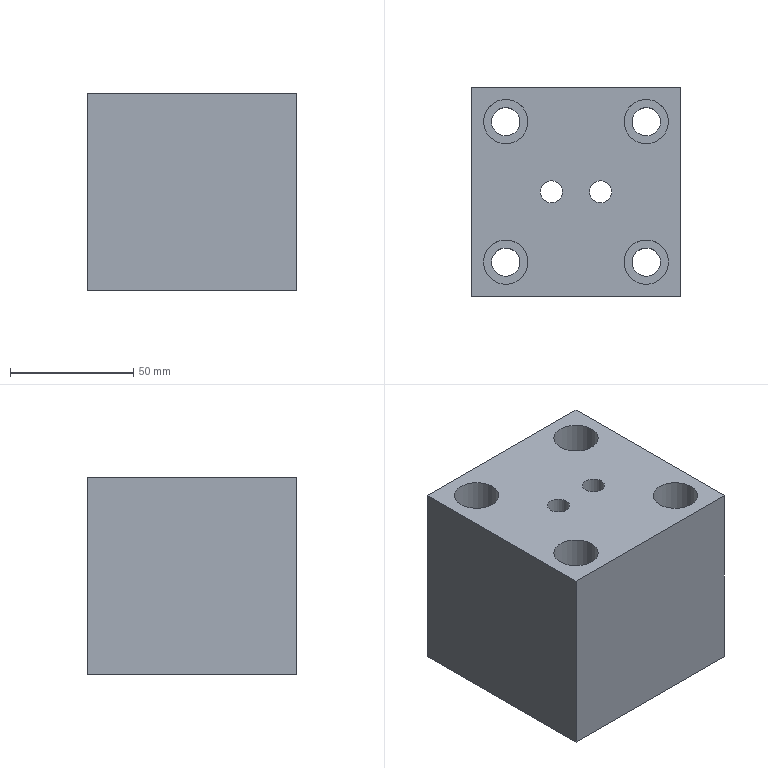Part | STEP file | lll_id4374_x_t | 1 solid | 24 faces | box 85 x 85 x 80 mm | volume 511038 mm3 | plane 12 | cylinder 12 | commonest cylinder face diameters 11.509 x4 18.008 x4 9 x2 14 x2
STEP:
#1=CARTESIAN_POINT('',(1584.69,-336.,-370.));
#2=VERTEX_POINT('',#1);
#3=CARTESIAN_POINT('',(1578.935,-336.,-370.));
#4=DIRECTION('',(0.,0.,1.));
#5=DIRECTION('',(1.,0.,0.));
#6=AXIS2_PLACEMENT_3D('',#3,#4,#5);
#7=CIRCLE('',#6,5.755);
#8=EDGE_CURVE('',#2,#2,#7,.T.);
#9=ORIENTED_EDGE('',*,*,#8,.T.);
#10=EDGE_LOOP('',(#9));
#11=FACE_BOUND('',#10,.T.);
#12=CARTESIAN_POINT('',(1584.69,-279.,-370.));
#13=VERTEX_POINT('',#12);
#14=CARTESIAN_POINT('',(1578.935,-279.,-370.));
#15=DIRECTION('',(0.,0.,1.));
#16=DIRECTION('',(1.,0.,0.));
#17=AXIS2_PLACEMENT_3D('',#14,#15,#16);
#18=CIRCLE('',#17,5.755);
#19=EDGE_CURVE('',#13,#13,#18,.T.);
#20=ORIENTED_EDGE('',*,*,#19,.T.);
#21=EDGE_LOOP('',(#20));
#22=FACE_BOUND('',#21,.T.);
#23=CARTESIAN_POINT('',(1527.69,-336.,-370.));
#24=VERTEX_POINT('',#23);
#25=CARTESIAN_POINT('',(1521.935,-336.,-370.));
#26=DIRECTION('',(0.,0.,1.));
#27=DIRECTION('',(1.,0.,0.));
#28=AXIS2_PLACEMENT_3D('',#25,#26,#27);
#29=CIRCLE('',#28,5.755);
#30=EDGE_CURVE('',#24,#24,#29,.T.);
#31=ORIENTED_EDGE('',*,*,#30,.T.);
#32=EDGE_LOOP('',(#31));
#33=FACE_BOUND('',#32,.T.);
#34=CARTESIAN_POINT('',(1527.69,-279.,-370.));
#35=VERTEX_POINT('',#34);
#36=CARTESIAN_POINT('',(1521.935,-279.,-370.));
#37=DIRECTION('',(0.,0.,1.));
#38=DIRECTION('',(1.,0.,0.));
#39=AXIS2_PLACEMENT_3D('',#36,#37,#38);
#40=CIRCLE('',#39,5.755);
#41=EDGE_CURVE('',#35,#35,#40,.T.);
#42=ORIENTED_EDGE('',*,*,#41,.T.);
#43=EDGE_LOOP('',(#42));
#44=FACE_BOUND('',#43,.T.);
#45=CARTESIAN_POINT('',(1592.935,-350.,-370.));
#46=VERTEX_POINT('',#45);
#47=CARTESIAN_POINT('',(1592.935,-265.,-370.));
#48=VERTEX_POINT('',#47);
#49=CARTESIAN_POINT('',(1592.935,0.,-370.));
#50=DIRECTION('',(0.,1.,0.));
#51=VECTOR('',#50,1.);
#52=LINE('',#49,#51);
#53=EDGE_CURVE('',#46,#48,#52,.T.);
#54=ORIENTED_EDGE('',*,*,#53,.F.);
#55=CARTESIAN_POINT('',(1507.935,-350.,-370.));
#56=VERTEX_POINT('',#55);
#57=CARTESIAN_POINT('',(1550.435,-350.,-370.));
#58=DIRECTION('',(-1.,0.,0.));
#59=VECTOR('',#58,1.);
#60=LINE('',#57,#59);
#61=EDGE_CURVE('',#46,#56,#60,.T.);
#62=ORIENTED_EDGE('',*,*,#61,.T.);
#63=CARTESIAN_POINT('',(1507.935,-265.,-370.));
#64=VERTEX_POINT('',#63);
#65=CARTESIAN_POINT('',(1507.935,0.,-370.));
#66=DIRECTION('',(0.,-1.,0.));
#67=VECTOR('',#66,1.);
#68=LINE('',#65,#67);
#69=EDGE_CURVE('',#64,#56,#68,.T.);
#70=ORIENTED_EDGE('',*,*,#69,.F.);
#71=CARTESIAN_POINT('',(2132.435,-265.,-370.));
#72=DIRECTION('',(-1.,0.,0.));
#73=VECTOR('',#72,1.);
#74=LINE('',#71,#73);
#75=EDGE_CURVE('',#48,#64,#74,.T.);
#76=ORIENTED_EDGE('',*,*,#75,.F.);
#77=EDGE_LOOP('',(#54,#62,#70,#76));
#78=FACE_BOUND('',#77,.T.);
#79=CARTESIAN_POINT('',(1567.435,-307.5,-370.));
#80=VERTEX_POINT('',#79);
#81=CARTESIAN_POINT('',(1560.435,-307.5,-370.));
#82=DIRECTION('',(0.,0.,1.));
#83=DIRECTION('',(1.,0.,0.));
#84=AXIS2_PLACEMENT_3D('',#81,#82,#83);
#85=CIRCLE('',#84,7.);
#86=EDGE_CURVE('',#80,#80,#85,.T.);
#87=ORIENTED_EDGE('',*,*,#86,.T.);
#88=EDGE_LOOP('',(#87));
#89=FACE_BOUND('',#88,.T.);
#90=CARTESIAN_POINT('',(1547.435,-307.5,-370.));
#91=VERTEX_POINT('',#90);
#92=CARTESIAN_POINT('',(1540.435,-307.5,-370.));
#93=DIRECTION('',(0.,0.,-1.));
#94=DIRECTION('',(1.,0.,0.));
#95=AXIS2_PLACEMENT_3D('',#92,#93,#94);
#96=CIRCLE('',#95,7.);
#97=EDGE_CURVE('',#91,#91,#96,.T.);
#98=ORIENTED_EDGE('',*,*,#97,.F.);
#99=EDGE_LOOP('',(#98));
#100=FACE_BOUND('',#99,.T.);
#101=CARTESIAN_POINT('',(2132.435,0.,-370.));
#102=DIRECTION('',(0.,0.,1.));
#103=DIRECTION('',(1.,0.,0.));
#104=AXIS2_PLACEMENT_3D('',#101,#102,#103);
#105=PLANE('',#104);
#106=ADVANCED_FACE('',(#11,#22,#33,#44,#78,#89,#100),#105,.F.);
#107=CARTESIAN_POINT('',(1535.935,-307.5,-290.));
#108=VERTEX_POINT('',#107);
#109=CARTESIAN_POINT('',(1540.435,-307.5,-290.));
#110=DIRECTION('',(0.,0.,-1.));
#111=DIRECTION('',(-1.,0.,0.));
#112=AXIS2_PLACEMENT_3D('',#109,#110,#111);
#113=CIRCLE('',#112,4.5);
#114=EDGE_CURVE('',#108,#108,#113,.T.);
#115=ORIENTED_EDGE('',*,*,#114,.F.);
#116=EDGE_LOOP('',(#115));
#117=FACE_BOUND('',#116,.T.);
#118=CARTESIAN_POINT('',(1535.935,-307.5,-300.));
#119=VERTEX_POINT('',#118);
#120=CARTESIAN_POINT('',(1540.435,-307.5,-300.));
#121=DIRECTION('',(0.,0.,-1.));
#122=DIRECTION('',(-1.,0.,0.));
#123=AXIS2_PLACEMENT_3D('',#120,#121,#122);
#124=CIRCLE('',#123,4.5);
#125=EDGE_CURVE('',#119,#119,#124,.T.);
#126=ORIENTED_EDGE('',*,*,#125,.T.);
#127=EDGE_LOOP('',(#126));
#128=FACE_BOUND('',#127,.T.);
#129=CARTESIAN_POINT('',(1540.435,-307.5,-510.));
#130=DIRECTION('',(0.,0.,1.));
#131=DIRECTION('',(1.,0.,0.));
#132=AXIS2_PLACEMENT_3D('',#129,#130,#131);
#133=CYLINDRICAL_SURFACE('',#132,4.5);
#134=ADVANCED_FACE('',(#117,#128),#133,.F.);
#135=ORIENTED_EDGE('',*,*,#114,.T.);
#136=EDGE_LOOP('',(#135));
#137=FACE_BOUND('',#136,.T.);
#138=CARTESIAN_POINT('',(1592.935,-265.,-290.));
#139=VERTEX_POINT('',#138);
#140=CARTESIAN_POINT('',(1592.935,-350.,-290.));
#141=VERTEX_POINT('',#140);
#142=CARTESIAN_POINT('',(1592.935,-87.5,-290.));
#143=DIRECTION('',(0.,-1.,0.));
#144=VECTOR('',#143,1.);
#145=LINE('',#142,#144);
#146=EDGE_CURVE('',#139,#141,#145,.T.);
#147=ORIENTED_EDGE('',*,*,#146,.F.);
#148=CARTESIAN_POINT('',(1507.935,-265.,-290.));
#149=VERTEX_POINT('',#148);
#150=CARTESIAN_POINT('',(1550.435,-265.,-290.));
#151=DIRECTION('',(-1.,0.,0.));
#152=VECTOR('',#151,1.);
#153=LINE('',#150,#152);
#154=EDGE_CURVE('',#139,#149,#153,.T.);
#155=ORIENTED_EDGE('',*,*,#154,.T.);
#156=CARTESIAN_POINT('',(1507.935,-350.,-290.));
#157=VERTEX_POINT('',#156);
#158=CARTESIAN_POINT('',(1507.935,-87.5,-290.));
#159=DIRECTION('',(0.,1.,0.));
#160=VECTOR('',#159,1.);
#161=LINE('',#158,#160);
#162=EDGE_CURVE('',#157,#149,#161,.T.);
#163=ORIENTED_EDGE('',*,*,#162,.F.);
#164=CARTESIAN_POINT('',(1550.435,-350.,-290.));
#165=DIRECTION('',(1.,0.,0.));
#166=VECTOR('',#165,1.);
#167=LINE('',#164,#166);
#168=EDGE_CURVE('',#157,#141,#167,.T.);
#169=ORIENTED_EDGE('',*,*,#168,.T.);
#170=EDGE_LOOP('',(#147,#155,#163,#169));
#171=FACE_BOUND('',#170,.T.);
#172=CARTESIAN_POINT('',(1512.931,-279.,-290.));
#173=VERTEX_POINT('',#172);
#174=CARTESIAN_POINT('',(1521.935,-279.,-290.));
#175=DIRECTION('',(0.,0.,-1.));
#176=DIRECTION('',(-1.,0.,0.));
#177=AXIS2_PLACEMENT_3D('',#174,#175,#176);
#178=CIRCLE('',#177,9.004);
#179=EDGE_CURVE('',#173,#173,#178,.T.);
#180=ORIENTED_EDGE('',*,*,#179,.T.);
#181=EDGE_LOOP('',(#180));
#182=FACE_BOUND('',#181,.T.);
#183=CARTESIAN_POINT('',(1512.931,-336.,-290.));
#184=VERTEX_POINT('',#183);
#185=CARTESIAN_POINT('',(1521.935,-336.,-290.));
#186=DIRECTION('',(0.,0.,-1.));
#187=DIRECTION('',(-1.,0.,0.));
#188=AXIS2_PLACEMENT_3D('',#185,#186,#187);
#189=CIRCLE('',#188,9.004);
#190=EDGE_CURVE('',#184,#184,#189,.T.);
#191=ORIENTED_EDGE('',*,*,#190,.T.);
#192=EDGE_LOOP('',(#191));
#193=FACE_BOUND('',#192,.T.);
#194=CARTESIAN_POINT('',(1569.931,-279.,-290.));
#195=VERTEX_POINT('',#194);
#196=CARTESIAN_POINT('',(1578.935,-279.,-290.));
#197=DIRECTION('',(0.,0.,-1.));
#198=DIRECTION('',(-1.,0.,0.));
#199=AXIS2_PLACEMENT_3D('',#196,#197,#198);
#200=CIRCLE('',#199,9.004);
#201=EDGE_CURVE('',#195,#195,#200,.T.);
#202=ORIENTED_EDGE('',*,*,#201,.T.);
#203=EDGE_LOOP('',(#202));
#204=FACE_BOUND('',#203,.T.);
#205=CARTESIAN_POINT('',(1569.931,-336.,-290.));
#206=VERTEX_POINT('',#205);
#207=CARTESIAN_POINT('',(1578.935,-336.,-290.));
#208=DIRECTION('',(0.,0.,-1.));
#209=DIRECTION('',(-1.,0.,0.));
#210=AXIS2_PLACEMENT_3D('',#207,#208,#209);
#211=CIRCLE('',#210,9.004);
#212=EDGE_CURVE('',#206,#206,#211,.T.);
#213=ORIENTED_EDGE('',*,*,#212,.T.);
#214=EDGE_LOOP('',(#213));
#215=FACE_BOUND('',#214,.T.);
#216=CARTESIAN_POINT('',(1555.935,-307.5,-290.));
#217=VERTEX_POINT('',#216);
#218=CARTESIAN_POINT('',(1560.435,-307.5,-290.));
#219=DIRECTION('',(0.,0.,1.));
#220=DIRECTION('',(-1.,0.,0.));
#221=AXIS2_PLACEMENT_3D('',#218,#219,#220);
#222=CIRCLE('',#221,4.5);
#223=EDGE_CURVE('',#217,#217,#222,.T.);
#224=ORIENTED_EDGE('',*,*,#223,.F.);
#225=EDGE_LOOP('',(#224));
#226=FACE_BOUND('',#225,.T.);
#227=CARTESIAN_POINT('',(1249.635,-87.5,-290.));
#228=DIRECTION('',(0.,0.,-1.));
#229=DIRECTION('',(-1.,0.,0.));
#230=AXIS2_PLACEMENT_3D('',#227,#228,#229);
#231=PLANE('',#230);
#232=ADVANCED_FACE('',(#137,#171,#182,#193,#204,#215,#226),#231,.F.);
#233=ORIENTED_EDGE('',*,*,#53,.T.);
#234=CARTESIAN_POINT('',(1592.935,-265.,-287.));
#235=DIRECTION('',(0.,0.,1.));
#236=VECTOR('',#235,1.);
#237=LINE('',#234,#236);
#238=EDGE_CURVE('',#48,#139,#237,.T.);
#239=ORIENTED_EDGE('',*,*,#238,.T.);
#240=ORIENTED_EDGE('',*,*,#146,.T.);
#241=CARTESIAN_POINT('',(1592.935,-350.,-287.));
#242=DIRECTION('',(0.,0.,1.));
#243=VECTOR('',#242,1.);
#244=LINE('',#241,#243);
#245=EDGE_CURVE('',#46,#141,#244,.T.);
#246=ORIENTED_EDGE('',*,*,#245,.F.);
#247=EDGE_LOOP('',(#233,#239,#240,#246));
#248=FACE_OUTER_BOUND('',#247,.T.);
#249=CARTESIAN_POINT('',(1592.935,-307.5,-287.));
#250=DIRECTION('',(1.,0.,0.));
#251=DIRECTION('',(0.,0.,-1.));
#252=AXIS2_PLACEMENT_3D('',#249,#250,#251);
#253=PLANE('',#252);
#254=ADVANCED_FACE('',(#248),#253,.T.);
#255=ORIENTED_EDGE('',*,*,#61,.F.);
#256=ORIENTED_EDGE('',*,*,#245,.T.);
#257=ORIENTED_EDGE('',*,*,#168,.F.);
#258=CARTESIAN_POINT('',(1507.935,-350.,-287.));
#259=DIRECTION('',(0.,0.,1.));
#260=VECTOR('',#259,1.);
#261=LINE('',#258,#260);
#262=EDGE_CURVE('',#56,#157,#261,.T.);
#263=ORIENTED_EDGE('',*,*,#262,.F.);
#264=EDGE_LOOP('',(#255,#256,#257,#263));
#265=FACE_OUTER_BOUND('',#264,.T.);
#266=CARTESIAN_POINT('',(1550.435,-350.,-287.));
#267=DIRECTION('',(0.,-1.,0.));
#268=DIRECTION('',(0.,0.,-1.));
#269=AXIS2_PLACEMENT_3D('',#266,#267,#268);
#270=PLANE('',#269);
#271=ADVANCED_FACE('',(#265),#270,.T.);
#272=ORIENTED_EDGE('',*,*,#69,.T.);
#273=ORIENTED_EDGE('',*,*,#262,.T.);
#274=ORIENTED_EDGE('',*,*,#162,.T.);
#275=CARTESIAN_POINT('',(1507.935,-265.,-287.));
#276=DIRECTION('',(0.,0.,1.));
#277=VECTOR('',#276,1.);
#278=LINE('',#275,#277);
#279=EDGE_CURVE('',#64,#149,#278,.T.);
#280=ORIENTED_EDGE('',*,*,#279,.F.);
#281=EDGE_LOOP('',(#272,#273,#274,#280));
#282=FACE_OUTER_BOUND('',#281,.T.);
#283=CARTESIAN_POINT('',(1507.935,-307.5,-287.));
#284=DIRECTION('',(-1.,0.,0.));
#285=DIRECTION('',(0.,0.,1.));
#286=AXIS2_PLACEMENT_3D('',#283,#284,#285);
#287=PLANE('',#286);
#288=ADVANCED_FACE('',(#282),#287,.T.);
#289=ORIENTED_EDGE('',*,*,#75,.T.);
#290=ORIENTED_EDGE('',*,*,#279,.T.);
#291=ORIENTED_EDGE('',*,*,#154,.F.);
#292=ORIENTED_EDGE('',*,*,#238,.F.);
#293=EDGE_LOOP('',(#289,#290,#291,#292));
#294=FACE_OUTER_BOUND('',#293,.T.);
#295=CARTESIAN_POINT('',(1550.435,-265.,-287.));
#296=DIRECTION('',(0.,1.,0.));
#297=DIRECTION('',(0.,0.,1.));
#298=AXIS2_PLACEMENT_3D('',#295,#296,#297);
#299=PLANE('',#298);
#300=ADVANCED_FACE('',(#294),#299,.T.);
#301=CARTESIAN_POINT('',(1516.181,-279.,-308.));
#302=VERTEX_POINT('',#301);
#303=CARTESIAN_POINT('',(1521.935,-279.,-308.));
#304=DIRECTION('',(0.,0.,-1.));
#305=DIRECTION('',(-1.,0.,0.));
#306=AXIS2_PLACEMENT_3D('',#303,#304,#305);
#307=CIRCLE('',#306,5.755);
#308=EDGE_CURVE('',#302,#302,#307,.T.);
#309=ORIENTED_EDGE('',*,*,#308,.F.);
#310=EDGE_LOOP('',(#309));
#311=FACE_BOUND('',#310,.T.);
#312=ORIENTED_EDGE('',*,*,#41,.F.);
#313=EDGE_LOOP('',(#312));
#314=FACE_BOUND('',#313,.T.);
#315=CARTESIAN_POINT('',(1521.935,-279.,-293.));
#316=DIRECTION('',(0.,0.,-1.));
#317=DIRECTION('',(1.,0.,0.));
#318=AXIS2_PLACEMENT_3D('',#315,#316,#317);
#319=CYLINDRICAL_SURFACE('',#318,5.755);
#320=ADVANCED_FACE('',(#311,#314),#319,.F.);
#321=ORIENTED_EDGE('',*,*,#308,.T.);
#322=EDGE_LOOP('',(#321));
#323=FACE_BOUND('',#322,.T.);
#324=CARTESIAN_POINT('',(1530.939,-279.,-308.));
#325=VERTEX_POINT('',#324);
#326=CARTESIAN_POINT('',(1521.935,-279.,-308.));
#327=DIRECTION('',(0.,0.,-1.));
#328=DIRECTION('',(1.,0.,0.));
#329=AXIS2_PLACEMENT_3D('',#326,#327,#328);
#330=CIRCLE('',#329,9.004);
#331=EDGE_CURVE('',#325,#325,#330,.T.);
#332=ORIENTED_EDGE('',*,*,#331,.F.);
#333=EDGE_LOOP('',(#332));
#334=FACE_BOUND('',#333,.T.);
#335=CARTESIAN_POINT('',(1521.935,-279.,-308.));
#336=DIRECTION('',(0.,0.,-1.));
#337=DIRECTION('',(-1.,0.,0.));
#338=AXIS2_PLACEMENT_3D('',#335,#336,#337);
#339=PLANE('',#338);
#340=ADVANCED_FACE('',(#323,#334),#339,.F.);
#341=ORIENTED_EDGE('',*,*,#331,.T.);
#342=EDGE_LOOP('',(#341));
#343=FACE_BOUND('',#342,.T.);
#344=ORIENTED_EDGE('',*,*,#179,.F.);
#345=EDGE_LOOP('',(#344));
#346=FACE_BOUND('',#345,.T.);
#347=CARTESIAN_POINT('',(1521.935,-279.,-295.));
#348=DIRECTION('',(0.,0.,-1.));
#349=DIRECTION('',(1.,0.,0.));
#350=AXIS2_PLACEMENT_3D('',#347,#348,#349);
#351=CYLINDRICAL_SURFACE('',#350,9.004);
#352=ADVANCED_FACE('',(#343,#346),#351,.F.);
#353=CARTESIAN_POINT('',(1516.181,-336.,-308.));
#354=VERTEX_POINT('',#353);
#355=CARTESIAN_POINT('',(1521.935,-336.,-308.));
#356=DIRECTION('',(0.,0.,-1.));
#357=DIRECTION('',(-1.,0.,0.));
#358=AXIS2_PLACEMENT_3D('',#355,#356,#357);
#359=CIRCLE('',#358,5.755);
#360=EDGE_CURVE('',#354,#354,#359,.T.);
#361=ORIENTED_EDGE('',*,*,#360,.F.);
#362=EDGE_LOOP('',(#361));
#363=FACE_BOUND('',#362,.T.);
#364=ORIENTED_EDGE('',*,*,#30,.F.);
#365=EDGE_LOOP('',(#364));
#366=FACE_BOUND('',#365,.T.);
#367=CARTESIAN_POINT('',(1521.935,-336.,-293.));
#368=DIRECTION('',(0.,0.,-1.));
#369=DIRECTION('',(1.,0.,0.));
#370=AXIS2_PLACEMENT_3D('',#367,#368,#369);
#371=CYLINDRICAL_SURFACE('',#370,5.755);
#372=ADVANCED_FACE('',(#363,#366),#371,.F.);
#373=ORIENTED_EDGE('',*,*,#360,.T.);
#374=EDGE_LOOP('',(#373));
#375=FACE_BOUND('',#374,.T.);
#376=CARTESIAN_POINT('',(1530.939,-336.,-308.));
#377=VERTEX_POINT('',#376);
#378=CARTESIAN_POINT('',(1521.935,-336.,-308.));
#379=DIRECTION('',(0.,0.,-1.));
#380=DIRECTION('',(1.,0.,0.));
#381=AXIS2_PLACEMENT_3D('',#378,#379,#380);
#382=CIRCLE('',#381,9.004);
#383=EDGE_CURVE('',#377,#377,#382,.T.);
#384=ORIENTED_EDGE('',*,*,#383,.F.);
#385=EDGE_LOOP('',(#384));
#386=FACE_BOUND('',#385,.T.);
#387=CARTESIAN_POINT('',(1521.935,-336.,-308.));
#388=DIRECTION('',(0.,0.,-1.));
#389=DIRECTION('',(-1.,0.,0.));
#390=AXIS2_PLACEMENT_3D('',#387,#388,#389);
#391=PLANE('',#390);
#392=ADVANCED_FACE('',(#375,#386),#391,.F.);
#393=ORIENTED_EDGE('',*,*,#383,.T.);
#394=EDGE_LOOP('',(#393));
#395=FACE_BOUND('',#394,.T.);
#396=ORIENTED_EDGE('',*,*,#190,.F.);
#397=EDGE_LOOP('',(#396));
#398=FACE_BOUND('',#397,.T.);
#399=CARTESIAN_POINT('',(1521.935,-336.,-295.));
#400=DIRECTION('',(0.,0.,-1.));
#401=DIRECTION('',(1.,0.,0.));
#402=AXIS2_PLACEMENT_3D('',#399,#400,#401);
#403=CYLINDRICAL_SURFACE('',#402,9.004);
#404=ADVANCED_FACE('',(#395,#398),#403,.F.);
#405=CARTESIAN_POINT('',(1573.181,-279.,-308.));
#406=VERTEX_POINT('',#405);
#407=CARTESIAN_POINT('',(1578.935,-279.,-308.));
#408=DIRECTION('',(0.,0.,-1.));
#409=DIRECTION('',(-1.,0.,0.));
#410=AXIS2_PLACEMENT_3D('',#407,#408,#409);
#411=CIRCLE('',#410,5.755);
#412=EDGE_CURVE('',#406,#406,#411,.T.);
#413=ORIENTED_EDGE('',*,*,#412,.F.);
#414=EDGE_LOOP('',(#413));
#415=FACE_BOUND('',#414,.T.);
#416=ORIENTED_EDGE('',*,*,#19,.F.);
#417=EDGE_LOOP('',(#416));
#418=FACE_BOUND('',#417,.T.);
#419=CARTESIAN_POINT('',(1578.935,-279.,-293.));
#420=DIRECTION('',(0.,0.,-1.));
#421=DIRECTION('',(1.,0.,0.));
#422=AXIS2_PLACEMENT_3D('',#419,#420,#421);
#423=CYLINDRICAL_SURFACE('',#422,5.755);
#424=ADVANCED_FACE('',(#415,#418),#423,.F.);
#425=ORIENTED_EDGE('',*,*,#412,.T.);
#426=EDGE_LOOP('',(#425));
#427=FACE_BOUND('',#426,.T.);
#428=CARTESIAN_POINT('',(1587.939,-279.,-308.));
#429=VERTEX_POINT('',#428);
#430=CARTESIAN_POINT('',(1578.935,-279.,-308.));
#431=DIRECTION('',(0.,0.,-1.));
#432=DIRECTION('',(1.,0.,0.));
#433=AXIS2_PLACEMENT_3D('',#430,#431,#432);
#434=CIRCLE('',#433,9.004);
#435=EDGE_CURVE('',#429,#429,#434,.T.);
#436=ORIENTED_EDGE('',*,*,#435,.F.);
#437=EDGE_LOOP('',(#436));
#438=FACE_BOUND('',#437,.T.);
#439=CARTESIAN_POINT('',(1578.935,-279.,-308.));
#440=DIRECTION('',(0.,0.,-1.));
#441=DIRECTION('',(-1.,0.,0.));
#442=AXIS2_PLACEMENT_3D('',#439,#440,#441);
#443=PLANE('',#442);
#444=ADVANCED_FACE('',(#427,#438),#443,.F.);
#445=ORIENTED_EDGE('',*,*,#435,.T.);
#446=EDGE_LOOP('',(#445));
#447=FACE_BOUND('',#446,.T.);
#448=ORIENTED_EDGE('',*,*,#201,.F.);
#449=EDGE_LOOP('',(#448));
#450=FACE_BOUND('',#449,.T.);
#451=CARTESIAN_POINT('',(1578.935,-279.,-295.));
#452=DIRECTION('',(0.,0.,-1.));
#453=DIRECTION('',(1.,0.,0.));
#454=AXIS2_PLACEMENT_3D('',#451,#452,#453);
#455=CYLINDRICAL_SURFACE('',#454,9.004);
#456=ADVANCED_FACE('',(#447,#450),#455,.F.);
#457=CARTESIAN_POINT('',(1573.181,-336.,-308.));
#458=VERTEX_POINT('',#457);
#459=CARTESIAN_POINT('',(1578.935,-336.,-308.));
#460=DIRECTION('',(0.,0.,-1.));
#461=DIRECTION('',(-1.,0.,0.));
#462=AXIS2_PLACEMENT_3D('',#459,#460,#461);
#463=CIRCLE('',#462,5.755);
#464=EDGE_CURVE('',#458,#458,#463,.T.);
#465=ORIENTED_EDGE('',*,*,#464,.F.);
#466=EDGE_LOOP('',(#465));
#467=FACE_BOUND('',#466,.T.);
#468=ORIENTED_EDGE('',*,*,#8,.F.);
#469=EDGE_LOOP('',(#468));
#470=FACE_BOUND('',#469,.T.);
#471=CARTESIAN_POINT('',(1578.935,-336.,-293.));
#472=DIRECTION('',(0.,0.,-1.));
#473=DIRECTION('',(1.,0.,0.));
#474=AXIS2_PLACEMENT_3D('',#471,#472,#473);
#475=CYLINDRICAL_SURFACE('',#474,5.755);
#476=ADVANCED_FACE('',(#467,#470),#475,.F.);
#477=ORIENTED_EDGE('',*,*,#464,.T.);
#478=EDGE_LOOP('',(#477));
#479=FACE_BOUND('',#478,.T.);
#480=CARTESIAN_POINT('',(1587.939,-336.,-308.));
#481=VERTEX_POINT('',#480);
#482=CARTESIAN_POINT('',(1578.935,-336.,-308.));
#483=DIRECTION('',(0.,0.,-1.));
#484=DIRECTION('',(1.,0.,0.));
#485=AXIS2_PLACEMENT_3D('',#482,#483,#484);
#486=CIRCLE('',#485,9.004);
#487=EDGE_CURVE('',#481,#481,#486,.T.);
#488=ORIENTED_EDGE('',*,*,#487,.F.);
#489=EDGE_LOOP('',(#488));
#490=FACE_BOUND('',#489,.T.);
#491=CARTESIAN_POINT('',(1578.935,-336.,-308.));
#492=DIRECTION('',(0.,0.,-1.));
#493=DIRECTION('',(-1.,0.,0.));
#494=AXIS2_PLACEMENT_3D('',#491,#492,#493);
#495=PLANE('',#494);
#496=ADVANCED_FACE('',(#479,#490),#495,.F.);
#497=ORIENTED_EDGE('',*,*,#487,.T.);
#498=EDGE_LOOP('',(#497));
#499=FACE_BOUND('',#498,.T.);
#500=ORIENTED_EDGE('',*,*,#212,.F.);
#501=EDGE_LOOP('',(#500));
#502=FACE_BOUND('',#501,.T.);
#503=CARTESIAN_POINT('',(1578.935,-336.,-295.));
#504=DIRECTION('',(0.,0.,-1.));
#505=DIRECTION('',(1.,0.,0.));
#506=AXIS2_PLACEMENT_3D('',#503,#504,#505);
#507=CYLINDRICAL_SURFACE('',#506,9.004);
#508=ADVANCED_FACE('',(#499,#502),#507,.F.);
#509=CARTESIAN_POINT('',(1564.935,-307.5,-300.));
#510=VERTEX_POINT('',#509);
#511=CARTESIAN_POINT('',(1560.435,-307.5,-300.));
#512=DIRECTION('',(0.,0.,-1.));
#513=DIRECTION('',(1.,0.,0.));
#514=AXIS2_PLACEMENT_3D('',#511,#512,#513);
#515=CIRCLE('',#514,4.5);
#516=EDGE_CURVE('',#510,#510,#515,.T.);
#517=ORIENTED_EDGE('',*,*,#516,.T.);
#518=EDGE_LOOP('',(#517));
#519=FACE_BOUND('',#518,.T.);
#520=ORIENTED_EDGE('',*,*,#223,.T.);
#521=EDGE_LOOP('',(#520));
#522=FACE_BOUND('',#521,.T.);
#523=CARTESIAN_POINT('',(1560.435,-307.5,-312.));
#524=DIRECTION('',(0.,0.,1.));
#525=DIRECTION('',(1.,0.,0.));
#526=AXIS2_PLACEMENT_3D('',#523,#524,#525);
#527=CYLINDRICAL_SURFACE('',#526,4.5);
#528=ADVANCED_FACE('',(#519,#522),#527,.F.);
#529=CARTESIAN_POINT('',(1567.435,-307.5,-300.));
#530=VERTEX_POINT('',#529);
#531=CARTESIAN_POINT('',(1560.435,-307.5,-300.));
#532=DIRECTION('',(0.,0.,-1.));
#533=DIRECTION('',(1.,0.,0.));
#534=AXIS2_PLACEMENT_3D('',#531,#532,#533);
#535=CIRCLE('',#534,7.);
#536=EDGE_CURVE('',#530,#530,#535,.T.);
#537=ORIENTED_EDGE('',*,*,#536,.F.);
#538=EDGE_LOOP('',(#537));
#539=FACE_BOUND('',#538,.T.);
#540=ORIENTED_EDGE('',*,*,#86,.F.);
#541=EDGE_LOOP('',(#540));
#542=FACE_BOUND('',#541,.T.);
#543=CARTESIAN_POINT('',(1560.435,-307.5,-510.));
#544=DIRECTION('',(0.,0.,1.));
#545=DIRECTION('',(1.,0.,0.));
#546=AXIS2_PLACEMENT_3D('',#543,#544,#545);
#547=CYLINDRICAL_SURFACE('',#546,7.);
#548=ADVANCED_FACE('',(#539,#542),#547,.F.);
#549=ORIENTED_EDGE('',*,*,#536,.T.);
#550=EDGE_LOOP('',(#549));
#551=FACE_BOUND('',#550,.T.);
#552=ORIENTED_EDGE('',*,*,#516,.F.);
#553=EDGE_LOOP('',(#552));
#554=FACE_BOUND('',#553,.T.);
#555=CARTESIAN_POINT('',(1560.435,-307.5,-300.));
#556=DIRECTION('',(0.,0.,1.));
#557=DIRECTION('',(1.,0.,0.));
#558=AXIS2_PLACEMENT_3D('',#555,#556,#557);
#559=PLANE('',#558);
#560=ADVANCED_FACE('',(#551,#554),#559,.F.);
#561=CARTESIAN_POINT('',(1533.435,-307.5,-300.));
#562=VERTEX_POINT('',#561);
#563=CARTESIAN_POINT('',(1540.435,-307.5,-300.));
#564=DIRECTION('',(0.,0.,1.));
#565=DIRECTION('',(-1.,0.,0.));
#566=AXIS2_PLACEMENT_3D('',#563,#564,#565);
#567=CIRCLE('',#566,7.);
#568=EDGE_CURVE('',#562,#562,#567,.T.);
#569=ORIENTED_EDGE('',*,*,#568,.T.);
#570=EDGE_LOOP('',(#569));
#571=FACE_BOUND('',#570,.T.);
#572=ORIENTED_EDGE('',*,*,#97,.T.);
#573=EDGE_LOOP('',(#572));
#574=FACE_BOUND('',#573,.T.);
#575=CARTESIAN_POINT('',(1540.435,-307.5,-510.));
#576=DIRECTION('',(0.,0.,1.));
#577=DIRECTION('',(1.,0.,0.));
#578=AXIS2_PLACEMENT_3D('',#575,#576,#577);
#579=CYLINDRICAL_SURFACE('',#578,7.);
#580=ADVANCED_FACE('',(#571,#574),#579,.F.);
#581=ORIENTED_EDGE('',*,*,#125,.F.);
#582=EDGE_LOOP('',(#581));
#583=FACE_BOUND('',#582,.T.);
#584=ORIENTED_EDGE('',*,*,#568,.F.);
#585=EDGE_LOOP('',(#584));
#586=FACE_BOUND('',#585,.T.);
#587=CARTESIAN_POINT('',(1540.435,-307.5,-300.));
#588=DIRECTION('',(0.,0.,-1.));
#589=DIRECTION('',(-1.,0.,0.));
#590=AXIS2_PLACEMENT_3D('',#587,#588,#589);
#591=PLANE('',#590);
#592=ADVANCED_FACE('',(#583,#586),#591,.T.);
#593=CLOSED_SHELL('',(#106,#134,#232,#254,#271,#288,#300,#320,#340,#352,#372,#392,#404,#424,#444,#456,#476,#496,#508,#528,#548,#560,#580,#592));
#594=MANIFOLD_SOLID_BREP('',#593);
#595=(LENGTH_UNIT()NAMED_UNIT(*)SI_UNIT(.MILLI.,.METRE.));
#596=UNCERTAINTY_MEASURE_WITH_UNIT(LENGTH_MEASURE(0.00002),#595,'','');
#597=(NAMED_UNIT(*)PLANE_ANGLE_UNIT()SI_UNIT($,.RADIAN.));
#598=PLANE_ANGLE_MEASURE_WITH_UNIT(PLANE_ANGLE_MEASURE(0.01745),#597);
#599=DIMENSIONAL_EXPONENTS(0.,0.,0.,0.,0.,0.,0.);
#600=(CONVERSION_BASED_UNIT('DEGREE',#598)NAMED_UNIT(#599)PLANE_ANGLE_UNIT());
#601=(NAMED_UNIT(*)SI_UNIT($,.STERADIAN.)SOLID_ANGLE_UNIT());
#602=(GEOMETRIC_REPRESENTATION_CONTEXT(3)GLOBAL_UNCERTAINTY_ASSIGNED_CONTEXT((#596))GLOBAL_UNIT_ASSIGNED_CONTEXT((#595,#600,#601))REPRESENTATION_CONTEXT('',''));
#603=ADVANCED_BREP_SHAPE_REPRESENTATION('',(#594),#602);